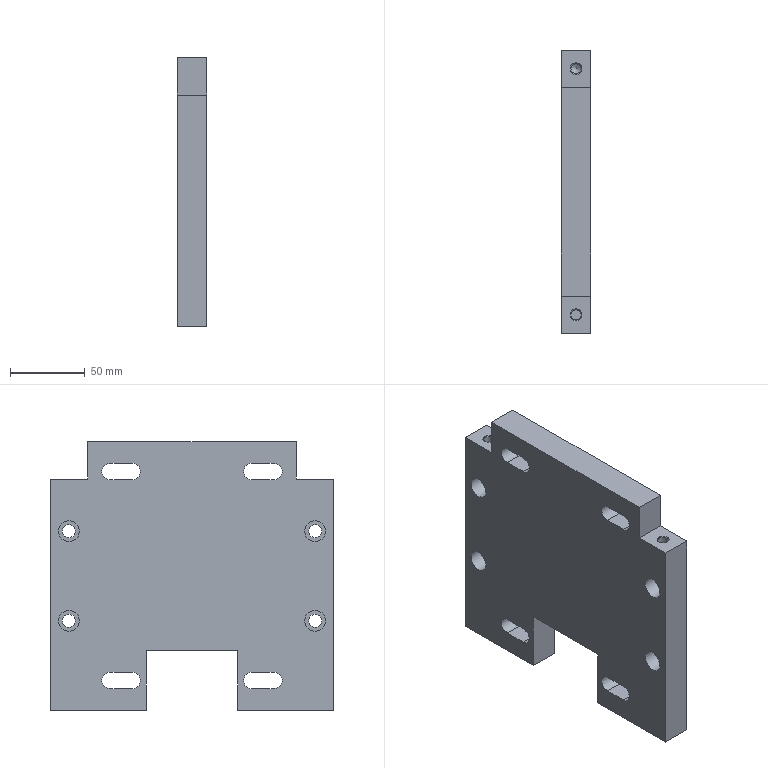Part | STEP file | 冲床-300配套压波_id982_x_t | 1 solid | 48 faces | box 20 x 190 x 180 mm | volume 579376 mm3 | plane 27 | cylinder 18 | cone 3 | commonest cylinder face diameters 11 x8 8.7 x4 14 x4 6.8 x2
STEP:
#1=CARTESIAN_POINT('',(1935.,-95.,-365.));
#2=VERTEX_POINT('',#1);
#3=CARTESIAN_POINT('',(1935.,-30.5,-365.));
#4=VERTEX_POINT('',#3);
#5=CARTESIAN_POINT('',(1935.,-100.,-365.));
#6=DIRECTION('',(0.,1.,0.));
#7=VECTOR('',#6,1.);
#8=LINE('',#5,#7);
#9=EDGE_CURVE('',#2,#4,#8,.T.);
#10=ORIENTED_EDGE('',*,*,#9,.T.);
#11=CARTESIAN_POINT('',(1955.,-30.5,-365.));
#12=VERTEX_POINT('',#11);
#13=CARTESIAN_POINT('',(1935.,-30.5,-365.));
#14=DIRECTION('',(1.,0.,0.));
#15=VECTOR('',#14,1.);
#16=LINE('',#13,#15);
#17=EDGE_CURVE('',#4,#12,#16,.T.);
#18=ORIENTED_EDGE('',*,*,#17,.T.);
#19=CARTESIAN_POINT('',(1955.,-95.,-365.));
#20=VERTEX_POINT('',#19);
#21=CARTESIAN_POINT('',(1955.,-100.,-365.));
#22=DIRECTION('',(0.,1.,0.));
#23=VECTOR('',#22,1.);
#24=LINE('',#21,#23);
#25=EDGE_CURVE('',#20,#12,#24,.T.);
#26=ORIENTED_EDGE('',*,*,#25,.F.);
#27=CARTESIAN_POINT('',(1935.,-95.,-365.));
#28=DIRECTION('',(1.,0.,0.));
#29=VECTOR('',#28,1.);
#30=LINE('',#27,#29);
#31=EDGE_CURVE('',#2,#20,#30,.T.);
#32=ORIENTED_EDGE('',*,*,#31,.F.);
#33=EDGE_LOOP('',(#10,#18,#26,#32));
#34=FACE_OUTER_BOUND('',#33,.T.);
#35=CARTESIAN_POINT('',(1935.,-100.,-365.));
#36=DIRECTION('',(0.,0.,-1.));
#37=DIRECTION('',(0.,1.,0.));
#38=AXIS2_PLACEMENT_3D('',#35,#36,#37);
#39=PLANE('',#38);
#40=ADVANCED_FACE('',(#34),#39,.T.);
#41=CARTESIAN_POINT('',(1941.6,-82.5,-230.));
#42=VERTEX_POINT('',#41);
#43=CARTESIAN_POINT('',(1945.,-82.5,-230.));
#44=DIRECTION('',(0.,0.,1.));
#45=DIRECTION('',(-1.,0.,0.));
#46=AXIS2_PLACEMENT_3D('',#43,#44,#45);
#47=CIRCLE('',#46,3.4);
#48=EDGE_CURVE('',#42,#42,#47,.T.);
#49=ORIENTED_EDGE('',*,*,#48,.T.);
#50=EDGE_LOOP('',(#49));
#51=FACE_OUTER_BOUND('',#50,.T.);
#52=CARTESIAN_POINT('',(1945.,-82.5,-230.));
#53=DIRECTION('',(0.,0.,-1.));
#54=DIRECTION('',(-1.,0.,0.));
#55=AXIS2_PLACEMENT_3D('',#52,#53,#54);
#56=PLANE('',#55);
#57=ADVANCED_FACE('',(#51),#56,.F.);
#58=CARTESIAN_POINT('',(1941.6,82.5,-230.));
#59=VERTEX_POINT('',#58);
#60=CARTESIAN_POINT('',(1945.,82.5,-230.));
#61=DIRECTION('',(0.,0.,1.));
#62=DIRECTION('',(-1.,0.,0.));
#63=AXIS2_PLACEMENT_3D('',#60,#61,#62);
#64=CIRCLE('',#63,3.4);
#65=EDGE_CURVE('',#59,#59,#64,.T.);
#66=ORIENTED_EDGE('',*,*,#65,.T.);
#67=EDGE_LOOP('',(#66));
#68=FACE_BOUND('',#67,.T.);
#69=CARTESIAN_POINT('',(1945.,82.5,-232.043));
#70=VERTEX_POINT('',#69);
#71=VERTEX_LOOP('',#70);
#72=FACE_BOUND('',#71,.T.);
#73=CARTESIAN_POINT('',(1945.,82.5,-230.));
#74=DIRECTION('',(0.,0.,1.));
#75=DIRECTION('',(1.,0.,0.));
#76=AXIS2_PLACEMENT_3D('',#73,#74,#75);
#77=CONICAL_SURFACE('',#76,3.4,59.);
#78=ADVANCED_FACE('',(#68,#72),#77,.F.);
#79=CARTESIAN_POINT('',(1941.6,-82.5,-210.6));
#80=VERTEX_POINT('',#79);
#81=CARTESIAN_POINT('',(1945.,-82.5,-210.6));
#82=DIRECTION('',(0.,0.,1.));
#83=DIRECTION('',(-1.,0.,0.));
#84=AXIS2_PLACEMENT_3D('',#81,#82,#83);
#85=CIRCLE('',#84,3.4);
#86=EDGE_CURVE('',#80,#80,#85,.T.);
#87=ORIENTED_EDGE('',*,*,#86,.T.);
#88=EDGE_LOOP('',(#87));
#89=FACE_BOUND('',#88,.T.);
#90=ORIENTED_EDGE('',*,*,#48,.F.);
#91=EDGE_LOOP('',(#90));
#92=FACE_BOUND('',#91,.T.);
#93=CARTESIAN_POINT('',(1945.,-82.5,-210.));
#94=DIRECTION('',(0.,0.,-1.));
#95=DIRECTION('',(-1.,0.,0.));
#96=AXIS2_PLACEMENT_3D('',#93,#94,#95);
#97=CYLINDRICAL_SURFACE('',#96,3.4);
#98=ADVANCED_FACE('',(#89,#92),#97,.F.);
#99=CARTESIAN_POINT('',(1941.6,82.5,-210.6));
#100=VERTEX_POINT('',#99);
#101=CARTESIAN_POINT('',(1945.,82.5,-210.6));
#102=DIRECTION('',(0.,0.,1.));
#103=DIRECTION('',(-1.,0.,0.));
#104=AXIS2_PLACEMENT_3D('',#101,#102,#103);
#105=CIRCLE('',#104,3.4);
#106=EDGE_CURVE('',#100,#100,#105,.T.);
#107=ORIENTED_EDGE('',*,*,#106,.T.);
#108=EDGE_LOOP('',(#107));
#109=FACE_BOUND('',#108,.T.);
#110=ORIENTED_EDGE('',*,*,#65,.F.);
#111=EDGE_LOOP('',(#110));
#112=FACE_BOUND('',#111,.T.);
#113=CARTESIAN_POINT('',(1945.,82.5,-210.));
#114=DIRECTION('',(0.,0.,-1.));
#115=DIRECTION('',(-1.,0.,0.));
#116=AXIS2_PLACEMENT_3D('',#113,#114,#115);
#117=CYLINDRICAL_SURFACE('',#116,3.4);
#118=ADVANCED_FACE('',(#109,#112),#117,.F.);
#119=ORIENTED_EDGE('',*,*,#86,.F.);
#120=EDGE_LOOP('',(#119));
#121=FACE_BOUND('',#120,.T.);
#122=CARTESIAN_POINT('',(1941.,-82.5,-210.));
#123=VERTEX_POINT('',#122);
#124=CARTESIAN_POINT('',(1945.,-82.5,-210.));
#125=DIRECTION('',(0.,0.,-1.));
#126=DIRECTION('',(-1.,0.,0.));
#127=AXIS2_PLACEMENT_3D('',#124,#125,#126);
#128=CIRCLE('',#127,4.);
#129=EDGE_CURVE('',#123,#123,#128,.T.);
#130=ORIENTED_EDGE('',*,*,#129,.F.);
#131=EDGE_LOOP('',(#130));
#132=FACE_BOUND('',#131,.T.);
#133=CARTESIAN_POINT('',(1945.,-82.5,-210.));
#134=DIRECTION('',(0.,0.,1.));
#135=DIRECTION('',(1.,0.,0.));
#136=AXIS2_PLACEMENT_3D('',#133,#134,#135);
#137=CONICAL_SURFACE('',#136,4.,45.);
#138=ADVANCED_FACE('',(#121,#132),#137,.F.);
#139=ORIENTED_EDGE('',*,*,#106,.F.);
#140=EDGE_LOOP('',(#139));
#141=FACE_BOUND('',#140,.T.);
#142=CARTESIAN_POINT('',(1941.,82.5,-210.));
#143=VERTEX_POINT('',#142);
#144=CARTESIAN_POINT('',(1945.,82.5,-210.));
#145=DIRECTION('',(0.,0.,-1.));
#146=DIRECTION('',(-1.,0.,0.));
#147=AXIS2_PLACEMENT_3D('',#144,#145,#146);
#148=CIRCLE('',#147,4.);
#149=EDGE_CURVE('',#143,#143,#148,.T.);
#150=ORIENTED_EDGE('',*,*,#149,.F.);
#151=EDGE_LOOP('',(#150));
#152=FACE_BOUND('',#151,.T.);
#153=CARTESIAN_POINT('',(1945.,82.5,-210.));
#154=DIRECTION('',(0.,0.,1.));
#155=DIRECTION('',(1.,0.,0.));
#156=AXIS2_PLACEMENT_3D('',#153,#154,#155);
#157=CONICAL_SURFACE('',#156,4.,45.);
#158=ADVANCED_FACE('',(#141,#152),#157,.F.);
#159=CARTESIAN_POINT('',(1945.,82.5,-249.35));
#160=VERTEX_POINT('',#159);
#161=CARTESIAN_POINT('',(1945.,82.5,-245.));
#162=DIRECTION('',(-1.,0.,0.));
#163=DIRECTION('',(0.,0.,-1.));
#164=AXIS2_PLACEMENT_3D('',#161,#162,#163);
#165=CIRCLE('',#164,4.35);
#166=EDGE_CURVE('',#160,#160,#165,.T.);
#167=ORIENTED_EDGE('',*,*,#166,.F.);
#168=EDGE_LOOP('',(#167));
#169=FACE_BOUND('',#168,.T.);
#170=CARTESIAN_POINT('',(1945.,82.5,-252.));
#171=VERTEX_POINT('',#170);
#172=CARTESIAN_POINT('',(1945.,82.5,-245.));
#173=DIRECTION('',(-1.,0.,0.));
#174=DIRECTION('',(0.,0.,-1.));
#175=AXIS2_PLACEMENT_3D('',#172,#173,#174);
#176=CIRCLE('',#175,7.);
#177=EDGE_CURVE('',#171,#171,#176,.T.);
#178=ORIENTED_EDGE('',*,*,#177,.T.);
#179=EDGE_LOOP('',(#178));
#180=FACE_BOUND('',#179,.T.);
#181=CARTESIAN_POINT('',(1945.,82.5,-245.));
#182=DIRECTION('',(1.,0.,0.));
#183=DIRECTION('',(0.,0.,-1.));
#184=AXIS2_PLACEMENT_3D('',#181,#182,#183);
#185=PLANE('',#184);
#186=ADVANCED_FACE('',(#169,#180),#185,.F.);
#187=CARTESIAN_POINT('',(1945.,82.5,-309.35));
#188=VERTEX_POINT('',#187);
#189=CARTESIAN_POINT('',(1945.,82.5,-305.));
#190=DIRECTION('',(-1.,0.,0.));
#191=DIRECTION('',(0.,0.,-1.));
#192=AXIS2_PLACEMENT_3D('',#189,#190,#191);
#193=CIRCLE('',#192,4.35);
#194=EDGE_CURVE('',#188,#188,#193,.T.);
#195=ORIENTED_EDGE('',*,*,#194,.F.);
#196=EDGE_LOOP('',(#195));
#197=FACE_BOUND('',#196,.T.);
#198=CARTESIAN_POINT('',(1945.,82.5,-312.));
#199=VERTEX_POINT('',#198);
#200=CARTESIAN_POINT('',(1945.,82.5,-305.));
#201=DIRECTION('',(-1.,0.,0.));
#202=DIRECTION('',(0.,0.,-1.));
#203=AXIS2_PLACEMENT_3D('',#200,#201,#202);
#204=CIRCLE('',#203,7.);
#205=EDGE_CURVE('',#199,#199,#204,.T.);
#206=ORIENTED_EDGE('',*,*,#205,.T.);
#207=EDGE_LOOP('',(#206));
#208=FACE_BOUND('',#207,.T.);
#209=CARTESIAN_POINT('',(1945.,82.5,-305.));
#210=DIRECTION('',(1.,0.,0.));
#211=DIRECTION('',(0.,0.,-1.));
#212=AXIS2_PLACEMENT_3D('',#209,#210,#211);
#213=PLANE('',#212);
#214=ADVANCED_FACE('',(#197,#208),#213,.F.);
#215=CARTESIAN_POINT('',(1945.,-82.5,-309.35));
#216=VERTEX_POINT('',#215);
#217=CARTESIAN_POINT('',(1945.,-82.5,-305.));
#218=DIRECTION('',(-1.,0.,0.));
#219=DIRECTION('',(0.,0.,-1.));
#220=AXIS2_PLACEMENT_3D('',#217,#218,#219);
#221=CIRCLE('',#220,4.35);
#222=EDGE_CURVE('',#216,#216,#221,.T.);
#223=ORIENTED_EDGE('',*,*,#222,.F.);
#224=EDGE_LOOP('',(#223));
#225=FACE_BOUND('',#224,.T.);
#226=CARTESIAN_POINT('',(1945.,-82.5,-312.));
#227=VERTEX_POINT('',#226);
#228=CARTESIAN_POINT('',(1945.,-82.5,-305.));
#229=DIRECTION('',(-1.,0.,0.));
#230=DIRECTION('',(0.,0.,-1.));
#231=AXIS2_PLACEMENT_3D('',#228,#229,#230);
#232=CIRCLE('',#231,7.);
#233=EDGE_CURVE('',#227,#227,#232,.T.);
#234=ORIENTED_EDGE('',*,*,#233,.T.);
#235=EDGE_LOOP('',(#234));
#236=FACE_BOUND('',#235,.T.);
#237=CARTESIAN_POINT('',(1945.,-82.5,-305.));
#238=DIRECTION('',(1.,0.,0.));
#239=DIRECTION('',(0.,0.,-1.));
#240=AXIS2_PLACEMENT_3D('',#237,#238,#239);
#241=PLANE('',#240);
#242=ADVANCED_FACE('',(#225,#236),#241,.F.);
#243=CARTESIAN_POINT('',(1945.,-82.5,-249.35));
#244=VERTEX_POINT('',#243);
#245=CARTESIAN_POINT('',(1945.,-82.5,-245.));
#246=DIRECTION('',(-1.,0.,0.));
#247=DIRECTION('',(0.,0.,-1.));
#248=AXIS2_PLACEMENT_3D('',#245,#246,#247);
#249=CIRCLE('',#248,4.35);
#250=EDGE_CURVE('',#244,#244,#249,.T.);
#251=ORIENTED_EDGE('',*,*,#250,.F.);
#252=EDGE_LOOP('',(#251));
#253=FACE_BOUND('',#252,.T.);
#254=CARTESIAN_POINT('',(1945.,-82.5,-252.));
#255=VERTEX_POINT('',#254);
#256=CARTESIAN_POINT('',(1945.,-82.5,-245.));
#257=DIRECTION('',(-1.,0.,0.));
#258=DIRECTION('',(0.,0.,-1.));
#259=AXIS2_PLACEMENT_3D('',#256,#257,#258);
#260=CIRCLE('',#259,7.);
#261=EDGE_CURVE('',#255,#255,#260,.T.);
#262=ORIENTED_EDGE('',*,*,#261,.T.);
#263=EDGE_LOOP('',(#262));
#264=FACE_BOUND('',#263,.T.);
#265=CARTESIAN_POINT('',(1945.,-82.5,-245.));
#266=DIRECTION('',(1.,0.,0.));
#267=DIRECTION('',(0.,0.,-1.));
#268=AXIS2_PLACEMENT_3D('',#265,#266,#267);
#269=PLANE('',#268);
#270=ADVANCED_FACE('',(#253,#264),#269,.F.);
#271=CARTESIAN_POINT('',(1955.,-40.,-339.5));
#272=VERTEX_POINT('',#271);
#273=CARTESIAN_POINT('',(1955.,-55.,-339.5));
#274=VERTEX_POINT('',#273);
#275=CARTESIAN_POINT('',(1955.,-100.,-339.5));
#276=DIRECTION('',(0.,-1.,0.));
#277=VECTOR('',#276,1.);
#278=LINE('',#275,#277);
#279=EDGE_CURVE('',#272,#274,#278,.T.);
#280=ORIENTED_EDGE('',*,*,#279,.T.);
#281=CARTESIAN_POINT('',(1935.,-55.,-339.5));
#282=VERTEX_POINT('',#281);
#283=CARTESIAN_POINT('',(1785.,-55.,-339.5));
#284=DIRECTION('',(-1.,0.,0.));
#285=VECTOR('',#284,1.);
#286=LINE('',#283,#285);
#287=EDGE_CURVE('',#274,#282,#286,.T.);
#288=ORIENTED_EDGE('',*,*,#287,.T.);
#289=CARTESIAN_POINT('',(1935.,-40.,-339.5));
#290=VERTEX_POINT('',#289);
#291=CARTESIAN_POINT('',(1935.,-100.,-339.5));
#292=DIRECTION('',(0.,-1.,0.));
#293=VECTOR('',#292,1.);
#294=LINE('',#291,#293);
#295=EDGE_CURVE('',#290,#282,#294,.T.);
#296=ORIENTED_EDGE('',*,*,#295,.F.);
#297=CARTESIAN_POINT('',(1785.,-40.,-339.5));
#298=DIRECTION('',(-1.,0.,0.));
#299=VECTOR('',#298,1.);
#300=LINE('',#297,#299);
#301=EDGE_CURVE('',#272,#290,#300,.T.);
#302=ORIENTED_EDGE('',*,*,#301,.F.);
#303=EDGE_LOOP('',(#280,#288,#296,#302));
#304=FACE_OUTER_BOUND('',#303,.T.);
#305=CARTESIAN_POINT('',(1785.,-30.,-339.5));
#306=DIRECTION('',(0.,0.,1.));
#307=DIRECTION('',(1.,0.,0.));
#308=AXIS2_PLACEMENT_3D('',#305,#306,#307);
#309=PLANE('',#308);
#310=ADVANCED_FACE('',(#304),#309,.F.);
#311=CARTESIAN_POINT('',(1955.,-55.,-350.5));
#312=VERTEX_POINT('',#311);
#313=CARTESIAN_POINT('',(1955.,-55.,-345.));
#314=DIRECTION('',(1.,0.,0.));
#315=DIRECTION('',(0.,0.,-1.));
#316=AXIS2_PLACEMENT_3D('',#313,#314,#315);
#317=CIRCLE('',#316,5.5);
#318=EDGE_CURVE('',#274,#312,#317,.T.);
#319=ORIENTED_EDGE('',*,*,#318,.T.);
#320=CARTESIAN_POINT('',(1935.,-55.,-350.5));
#321=VERTEX_POINT('',#320);
#322=CARTESIAN_POINT('',(1785.,-55.,-350.5));
#323=DIRECTION('',(-1.,0.,0.));
#324=VECTOR('',#323,1.);
#325=LINE('',#322,#324);
#326=EDGE_CURVE('',#312,#321,#325,.T.);
#327=ORIENTED_EDGE('',*,*,#326,.T.);
#328=CARTESIAN_POINT('',(1935.,-55.,-345.));
#329=DIRECTION('',(1.,0.,0.));
#330=DIRECTION('',(0.,0.,-1.));
#331=AXIS2_PLACEMENT_3D('',#328,#329,#330);
#332=CIRCLE('',#331,5.5);
#333=EDGE_CURVE('',#282,#321,#332,.T.);
#334=ORIENTED_EDGE('',*,*,#333,.F.);
#335=ORIENTED_EDGE('',*,*,#287,.F.);
#336=EDGE_LOOP('',(#319,#327,#334,#335));
#337=FACE_OUTER_BOUND('',#336,.T.);
#338=CARTESIAN_POINT('',(1785.,-55.,-345.));
#339=DIRECTION('',(1.,0.,0.));
#340=DIRECTION('',(0.,0.,-1.));
#341=AXIS2_PLACEMENT_3D('',#338,#339,#340);
#342=CYLINDRICAL_SURFACE('',#341,5.5);
#343=ADVANCED_FACE('',(#337),#342,.F.);
#344=CARTESIAN_POINT('',(1955.,-40.,-350.5));
#345=VERTEX_POINT('',#344);
#346=CARTESIAN_POINT('',(1955.,-100.,-350.5));
#347=DIRECTION('',(0.,-1.,0.));
#348=VECTOR('',#347,1.);
#349=LINE('',#346,#348);
#350=EDGE_CURVE('',#345,#312,#349,.T.);
#351=ORIENTED_EDGE('',*,*,#350,.F.);
#352=CARTESIAN_POINT('',(1935.,-40.,-350.5));
#353=VERTEX_POINT('',#352);
#354=CARTESIAN_POINT('',(1785.,-40.,-350.5));
#355=DIRECTION('',(-1.,0.,0.));
#356=VECTOR('',#355,1.);
#357=LINE('',#354,#356);
#358=EDGE_CURVE('',#345,#353,#357,.T.);
#359=ORIENTED_EDGE('',*,*,#358,.T.);
#360=CARTESIAN_POINT('',(1935.,-100.,-350.5));
#361=DIRECTION('',(0.,1.,0.));
#362=VECTOR('',#361,1.);
#363=LINE('',#360,#362);
#364=EDGE_CURVE('',#321,#353,#363,.T.);
#365=ORIENTED_EDGE('',*,*,#364,.F.);
#366=ORIENTED_EDGE('',*,*,#326,.F.);
#367=EDGE_LOOP('',(#351,#359,#365,#366));
#368=FACE_OUTER_BOUND('',#367,.T.);
#369=CARTESIAN_POINT('',(1785.,-70.,-350.5));
#370=DIRECTION('',(0.,0.,-1.));
#371=DIRECTION('',(-1.,0.,0.));
#372=AXIS2_PLACEMENT_3D('',#369,#370,#371);
#373=PLANE('',#372);
#374=ADVANCED_FACE('',(#368),#373,.F.);
#375=CARTESIAN_POINT('',(1955.,-40.,-345.));
#376=DIRECTION('',(1.,0.,0.));
#377=DIRECTION('',(0.,0.,-1.));
#378=AXIS2_PLACEMENT_3D('',#375,#376,#377);
#379=CIRCLE('',#378,5.5);
#380=EDGE_CURVE('',#345,#272,#379,.T.);
#381=ORIENTED_EDGE('',*,*,#380,.T.);
#382=ORIENTED_EDGE('',*,*,#301,.T.);
#383=CARTESIAN_POINT('',(1935.,-40.,-345.));
#384=DIRECTION('',(1.,0.,0.));
#385=DIRECTION('',(0.,0.,-1.));
#386=AXIS2_PLACEMENT_3D('',#383,#384,#385);
#387=CIRCLE('',#386,5.5);
#388=EDGE_CURVE('',#353,#290,#387,.T.);
#389=ORIENTED_EDGE('',*,*,#388,.F.);
#390=ORIENTED_EDGE('',*,*,#358,.F.);
#391=EDGE_LOOP('',(#381,#382,#389,#390));
#392=FACE_OUTER_BOUND('',#391,.T.);
#393=CARTESIAN_POINT('',(1785.,-40.,-345.));
#394=DIRECTION('',(1.,0.,0.));
#395=DIRECTION('',(0.,0.,-1.));
#396=AXIS2_PLACEMENT_3D('',#393,#394,#395);
#397=CYLINDRICAL_SURFACE('',#396,5.5);
#398=ADVANCED_FACE('',(#392),#397,.F.);
#399=CARTESIAN_POINT('',(1955.,55.,-210.5));
#400=VERTEX_POINT('',#399);
#401=CARTESIAN_POINT('',(1955.,55.,-199.5));
#402=VERTEX_POINT('',#401);
#403=CARTESIAN_POINT('',(1955.,55.,-205.));
#404=DIRECTION('',(1.,0.,0.));
#405=DIRECTION('',(0.,0.,-1.));
#406=AXIS2_PLACEMENT_3D('',#403,#404,#405);
#407=CIRCLE('',#406,5.5);
#408=EDGE_CURVE('',#400,#402,#407,.T.);
#409=ORIENTED_EDGE('',*,*,#408,.T.);
#410=CARTESIAN_POINT('',(1935.,55.,-199.5));
#411=VERTEX_POINT('',#410);
#412=CARTESIAN_POINT('',(1785.,55.,-199.5));
#413=DIRECTION('',(-1.,0.,0.));
#414=VECTOR('',#413,1.);
#415=LINE('',#412,#414);
#416=EDGE_CURVE('',#402,#411,#415,.T.);
#417=ORIENTED_EDGE('',*,*,#416,.T.);
#418=CARTESIAN_POINT('',(1935.,55.,-210.5));
#419=VERTEX_POINT('',#418);
#420=CARTESIAN_POINT('',(1935.,55.,-205.));
#421=DIRECTION('',(1.,0.,0.));
#422=DIRECTION('',(0.,0.,-1.));
#423=AXIS2_PLACEMENT_3D('',#420,#421,#422);
#424=CIRCLE('',#423,5.5);
#425=EDGE_CURVE('',#419,#411,#424,.T.);
#426=ORIENTED_EDGE('',*,*,#425,.F.);
#427=CARTESIAN_POINT('',(1785.,55.,-210.5));
#428=DIRECTION('',(-1.,0.,0.));
#429=VECTOR('',#428,1.);
#430=LINE('',#427,#429);
#431=EDGE_CURVE('',#400,#419,#430,.T.);
#432=ORIENTED_EDGE('',*,*,#431,.F.);
#433=EDGE_LOOP('',(#409,#417,#426,#432));
#434=FACE_OUTER_BOUND('',#433,.T.);
#435=CARTESIAN_POINT('',(1785.,55.,-205.));
#436=DIRECTION('',(1.,0.,0.));
#437=DIRECTION('',(0.,0.,1.));
#438=AXIS2_PLACEMENT_3D('',#435,#436,#437);
#439=CYLINDRICAL_SURFACE('',#438,5.5);
#440=ADVANCED_FACE('',(#434),#439,.F.);
#441=CARTESIAN_POINT('',(1955.,40.,-199.5));
#442=VERTEX_POINT('',#441);
#443=CARTESIAN_POINT('',(1955.,-100.,-199.5));
#444=DIRECTION('',(0.,-1.,0.));
#445=VECTOR('',#444,1.);
#446=LINE('',#443,#445);
#447=EDGE_CURVE('',#402,#442,#446,.T.);
#448=ORIENTED_EDGE('',*,*,#447,.T.);
#449=CARTESIAN_POINT('',(1935.,40.,-199.5));
#450=VERTEX_POINT('',#449);
#451=CARTESIAN_POINT('',(1785.,40.,-199.5));
#452=DIRECTION('',(-1.,0.,0.));
#453=VECTOR('',#452,1.);
#454=LINE('',#451,#453);
#455=EDGE_CURVE('',#442,#450,#454,.T.);
#456=ORIENTED_EDGE('',*,*,#455,.T.);
#457=CARTESIAN_POINT('',(1935.,-100.,-199.5));
#458=DIRECTION('',(0.,-1.,0.));
#459=VECTOR('',#458,1.);
#460=LINE('',#457,#459);
#461=EDGE_CURVE('',#411,#450,#460,.T.);
#462=ORIENTED_EDGE('',*,*,#461,.F.);
#463=ORIENTED_EDGE('',*,*,#416,.F.);
#464=EDGE_LOOP('',(#448,#456,#462,#463));
#465=FACE_OUTER_BOUND('',#464,.T.);
#466=CARTESIAN_POINT('',(1785.,70.,-199.5));
#467=DIRECTION('',(0.,0.,1.));
#468=DIRECTION('',(-1.,0.,0.));
#469=AXIS2_PLACEMENT_3D('',#466,#467,#468);
#470=PLANE('',#469);
#471=ADVANCED_FACE('',(#465),#470,.F.);
#472=CARTESIAN_POINT('',(1955.,40.,-210.5));
#473=VERTEX_POINT('',#472);
#474=CARTESIAN_POINT('',(1955.,40.,-205.));
#475=DIRECTION('',(-1.,0.,0.));
#476=DIRECTION('',(0.,0.,-1.));
#477=AXIS2_PLACEMENT_3D('',#474,#475,#476);
#478=CIRCLE('',#477,5.5);
#479=EDGE_CURVE('',#473,#442,#478,.T.);
#480=ORIENTED_EDGE('',*,*,#479,.F.);
#481=CARTESIAN_POINT('',(1935.,40.,-210.5));
#482=VERTEX_POINT('',#481);
#483=CARTESIAN_POINT('',(1785.,40.,-210.5));
#484=DIRECTION('',(-1.,0.,0.));
#485=VECTOR('',#484,1.);
#486=LINE('',#483,#485);
#487=EDGE_CURVE('',#473,#482,#486,.T.);
#488=ORIENTED_EDGE('',*,*,#487,.T.);
#489=CARTESIAN_POINT('',(1935.,40.,-205.));
#490=DIRECTION('',(1.,0.,0.));
#491=DIRECTION('',(0.,0.,-1.));
#492=AXIS2_PLACEMENT_3D('',#489,#490,#491);
#493=CIRCLE('',#492,5.5);
#494=EDGE_CURVE('',#450,#482,#493,.T.);
#495=ORIENTED_EDGE('',*,*,#494,.F.);
#496=ORIENTED_EDGE('',*,*,#455,.F.);
#497=EDGE_LOOP('',(#480,#488,#495,#496));
#498=FACE_OUTER_BOUND('',#497,.T.);
#499=CARTESIAN_POINT('',(1785.,40.,-205.));
#500=DIRECTION('',(1.,0.,0.));
#501=DIRECTION('',(0.,0.,1.));
#502=AXIS2_PLACEMENT_3D('',#499,#500,#501);
#503=CYLINDRICAL_SURFACE('',#502,5.5);
#504=ADVANCED_FACE('',(#498),#503,.F.);
#505=CARTESIAN_POINT('',(1955.,-100.,-210.5));
#506=DIRECTION('',(0.,1.,0.));
#507=VECTOR('',#506,1.);
#508=LINE('',#505,#507);
#509=EDGE_CURVE('',#473,#400,#508,.T.);
#510=ORIENTED_EDGE('',*,*,#509,.T.);
#511=ORIENTED_EDGE('',*,*,#431,.T.);
#512=CARTESIAN_POINT('',(1935.,-100.,-210.5));
#513=DIRECTION('',(0.,1.,0.));
#514=VECTOR('',#513,1.);
#515=LINE('',#512,#514);
#516=EDGE_CURVE('',#482,#419,#515,.T.);
#517=ORIENTED_EDGE('',*,*,#516,.F.);
#518=ORIENTED_EDGE('',*,*,#487,.F.);
#519=EDGE_LOOP('',(#510,#511,#517,#518));
#520=FACE_OUTER_BOUND('',#519,.T.);
#521=CARTESIAN_POINT('',(1785.,30.,-210.5));
#522=DIRECTION('',(0.,0.,-1.));
#523=DIRECTION('',(1.,0.,0.));
#524=AXIS2_PLACEMENT_3D('',#521,#522,#523);
#525=PLANE('',#524);
#526=ADVANCED_FACE('',(#520),#525,.F.);
#527=CARTESIAN_POINT('',(1955.,-55.,-210.5));
#528=VERTEX_POINT('',#527);
#529=CARTESIAN_POINT('',(1955.,-40.,-210.5));
#530=VERTEX_POINT('',#529);
#531=CARTESIAN_POINT('',(1955.,-100.,-210.5));
#532=DIRECTION('',(0.,1.,0.));
#533=VECTOR('',#532,1.);
#534=LINE('',#531,#533);
#535=EDGE_CURVE('',#528,#530,#534,.T.);
#536=ORIENTED_EDGE('',*,*,#535,.T.);
#537=CARTESIAN_POINT('',(1935.,-40.,-210.5));
#538=VERTEX_POINT('',#537);
#539=CARTESIAN_POINT('',(1785.,-40.,-210.5));
#540=DIRECTION('',(1.,0.,0.));
#541=VECTOR('',#540,1.);
#542=LINE('',#539,#541);
#543=EDGE_CURVE('',#538,#530,#542,.T.);
#544=ORIENTED_EDGE('',*,*,#543,.F.);
#545=CARTESIAN_POINT('',(1935.,-55.,-210.5));
#546=VERTEX_POINT('',#545);
#547=CARTESIAN_POINT('',(1935.,-100.,-210.5));
#548=DIRECTION('',(0.,1.,0.));
#549=VECTOR('',#548,1.);
#550=LINE('',#547,#549);
#551=EDGE_CURVE('',#546,#538,#550,.T.);
#552=ORIENTED_EDGE('',*,*,#551,.F.);
#553=CARTESIAN_POINT('',(1785.,-55.,-210.5));
#554=DIRECTION('',(1.,0.,0.));
#555=VECTOR('',#554,1.);
#556=LINE('',#553,#555);
#557=EDGE_CURVE('',#546,#528,#556,.T.);
#558=ORIENTED_EDGE('',*,*,#557,.T.);
#559=EDGE_LOOP('',(#536,#544,#552,#558));
#560=FACE_OUTER_BOUND('',#559,.T.);
#561=CARTESIAN_POINT('',(1785.,-30.,-210.5));
#562=DIRECTION('',(0.,0.,-1.));
#563=DIRECTION('',(1.,0.,0.));
#564=AXIS2_PLACEMENT_3D('',#561,#562,#563);
#565=PLANE('',#564);
#566=ADVANCED_FACE('',(#560),#565,.F.);
#567=CARTESIAN_POINT('',(1955.,-40.,-199.5));
#568=VERTEX_POINT('',#567);
#569=CARTESIAN_POINT('',(1955.,-40.,-205.));
#570=DIRECTION('',(1.,0.,0.));
#571=DIRECTION('',(0.,0.,-1.));
#572=AXIS2_PLACEMENT_3D('',#569,#570,#571);
#573=CIRCLE('',#572,5.5);
#574=EDGE_CURVE('',#530,#568,#573,.T.);
#575=ORIENTED_EDGE('',*,*,#574,.T.);
#576=CARTESIAN_POINT('',(1935.,-40.,-199.5));
#577=VERTEX_POINT('',#576);
#578=CARTESIAN_POINT('',(1785.,-40.,-199.5));
#579=DIRECTION('',(1.,0.,0.));
#580=VECTOR('',#579,1.);
#581=LINE('',#578,#580);
#582=EDGE_CURVE('',#577,#568,#581,.T.);
#583=ORIENTED_EDGE('',*,*,#582,.F.);
#584=CARTESIAN_POINT('',(1935.,-40.,-205.));
#585=DIRECTION('',(1.,0.,0.));
#586=DIRECTION('',(0.,0.,-1.));
#587=AXIS2_PLACEMENT_3D('',#584,#585,#586);
#588=CIRCLE('',#587,5.5);
#589=EDGE_CURVE('',#538,#577,#588,.T.);
#590=ORIENTED_EDGE('',*,*,#589,.F.);
#591=ORIENTED_EDGE('',*,*,#543,.T.);
#592=EDGE_LOOP('',(#575,#583,#590,#591));
#593=FACE_OUTER_BOUND('',#592,.T.);
#594=CARTESIAN_POINT('',(1785.,-40.,-205.));
#595=DIRECTION('',(1.,0.,0.));
#596=DIRECTION('',(0.,0.,1.));
#597=AXIS2_PLACEMENT_3D('',#594,#595,#596);
#598=CYLINDRICAL_SURFACE('',#597,5.5);
#599=ADVANCED_FACE('',(#593),#598,.F.);
#600=CARTESIAN_POINT('',(1955.,-55.,-199.5));
#601=VERTEX_POINT('',#600);
#602=CARTESIAN_POINT('',(1955.,-100.,-199.5));
#603=DIRECTION('',(0.,1.,0.));
#604=VECTOR('',#603,1.);
#605=LINE('',#602,#604);
#606=EDGE_CURVE('',#601,#568,#605,.T.);
#607=ORIENTED_EDGE('',*,*,#606,.F.);
#608=CARTESIAN_POINT('',(1935.,-55.,-199.5));
#609=VERTEX_POINT('',#608);
#610=CARTESIAN_POINT('',(1785.,-55.,-199.5));
#611=DIRECTION('',(1.,0.,0.));
#612=VECTOR('',#611,1.);
#613=LINE('',#610,#612);
#614=EDGE_CURVE('',#609,#601,#613,.T.);
#615=ORIENTED_EDGE('',*,*,#614,.F.);
#616=CARTESIAN_POINT('',(1935.,-100.,-199.5));
#617=DIRECTION('',(0.,-1.,0.));
#618=VECTOR('',#617,1.);
#619=LINE('',#616,#618);
#620=EDGE_CURVE('',#577,#609,#619,.T.);
#621=ORIENTED_EDGE('',*,*,#620,.F.);
#622=ORIENTED_EDGE('',*,*,#582,.T.);
#623=EDGE_LOOP('',(#607,#615,#621,#622));
#624=FACE_OUTER_BOUND('',#623,.T.);
#625=CARTESIAN_POINT('',(1785.,-70.,-199.5));
#626=DIRECTION('',(0.,0.,1.));
#627=DIRECTION('',(-1.,0.,0.));
#628=AXIS2_PLACEMENT_3D('',#625,#626,#627);
#629=PLANE('',#628);
#630=ADVANCED_FACE('',(#624),#629,.F.);
#631=CARTESIAN_POINT('',(1955.,-55.,-205.));
#632=DIRECTION('',(1.,0.,0.));
#633=DIRECTION('',(0.,0.,-1.));
#634=AXIS2_PLACEMENT_3D('',#631,#632,#633);
#635=CIRCLE('',#634,5.5);
#636=EDGE_CURVE('',#601,#528,#635,.T.);
#637=ORIENTED_EDGE('',*,*,#636,.T.);
#638=ORIENTED_EDGE('',*,*,#557,.F.);
#639=CARTESIAN_POINT('',(1935.,-55.,-205.));
#640=DIRECTION('',(1.,0.,0.));
#641=DIRECTION('',(0.,0.,-1.));
#642=AXIS2_PLACEMENT_3D('',#639,#640,#641);
#643=CIRCLE('',#642,5.5);
#644=EDGE_CURVE('',#609,#546,#643,.T.);
#645=ORIENTED_EDGE('',*,*,#644,.F.);
#646=ORIENTED_EDGE('',*,*,#614,.T.);
#647=EDGE_LOOP('',(#637,#638,#645,#646));
#648=FACE_OUTER_BOUND('',#647,.T.);
#649=CARTESIAN_POINT('',(1785.,-55.,-205.));
#650=DIRECTION('',(1.,0.,0.));
#651=DIRECTION('',(0.,0.,1.));
#652=AXIS2_PLACEMENT_3D('',#649,#650,#651);
#653=CYLINDRICAL_SURFACE('',#652,5.5);
#654=ADVANCED_FACE('',(#648),#653,.F.);
#655=ORIENTED_EDGE('',*,*,#129,.T.);
#656=EDGE_LOOP('',(#655));
#657=FACE_BOUND('',#656,.T.);
#658=CARTESIAN_POINT('',(1935.,-70.,-210.));
#659=VERTEX_POINT('',#658);
#660=CARTESIAN_POINT('',(1935.,-95.,-210.));
#661=VERTEX_POINT('',#660);
#662=CARTESIAN_POINT('',(1935.,-70.,-210.));
#663=DIRECTION('',(0.,-1.,0.));
#664=VECTOR('',#663,1.);
#665=LINE('',#662,#664);
#666=EDGE_CURVE('',#659,#661,#665,.T.);
#667=ORIENTED_EDGE('',*,*,#666,.T.);
#668=CARTESIAN_POINT('',(1955.,-95.,-210.));
#669=VERTEX_POINT('',#668);
#670=CARTESIAN_POINT('',(1935.,-95.,-210.));
#671=DIRECTION('',(-1.,0.,0.));
#672=VECTOR('',#671,1.);
#673=LINE('',#670,#672);
#674=EDGE_CURVE('',#669,#661,#673,.T.);
#675=ORIENTED_EDGE('',*,*,#674,.F.);
#676=CARTESIAN_POINT('',(1955.,-70.,-210.));
#677=VERTEX_POINT('',#676);
#678=CARTESIAN_POINT('',(1955.,-70.,-210.));
#679=DIRECTION('',(0.,-1.,0.));
#680=VECTOR('',#679,1.);
#681=LINE('',#678,#680);
#682=EDGE_CURVE('',#677,#669,#681,.T.);
#683=ORIENTED_EDGE('',*,*,#682,.F.);
#684=CARTESIAN_POINT('',(1955.,-70.,-210.));
#685=DIRECTION('',(-1.,0.,0.));
#686=VECTOR('',#685,1.);
#687=LINE('',#684,#686);
#688=EDGE_CURVE('',#677,#659,#687,.T.);
#689=ORIENTED_EDGE('',*,*,#688,.T.);
#690=EDGE_LOOP('',(#667,#675,#683,#689));
#691=FACE_BOUND('',#690,.T.);
#692=CARTESIAN_POINT('',(1955.,-70.,-210.));
#693=DIRECTION('',(0.,0.,-1.));
#694=DIRECTION('',(-1.,0.,0.));
#695=AXIS2_PLACEMENT_3D('',#692,#693,#694);
#696=PLANE('',#695);
#697=ADVANCED_FACE('',(#657,#691),#696,.F.);
#698=CARTESIAN_POINT('',(1955.,-70.,-185.));
#699=VERTEX_POINT('',#698);
#700=CARTESIAN_POINT('',(1935.,-70.,-185.));
#701=VERTEX_POINT('',#700);
#702=CARTESIAN_POINT('',(1935.,-70.,-185.));
#703=DIRECTION('',(-1.,0.,0.));
#704=VECTOR('',#703,1.);
#705=LINE('',#702,#704);
#706=EDGE_CURVE('',#699,#701,#705,.T.);
#707=ORIENTED_EDGE('',*,*,#706,.T.);
#708=CARTESIAN_POINT('',(1935.,-70.,-180.));
#709=DIRECTION('',(0.,0.,-1.));
#710=VECTOR('',#709,1.);
#711=LINE('',#708,#710);
#712=EDGE_CURVE('',#701,#659,#711,.T.);
#713=ORIENTED_EDGE('',*,*,#712,.T.);
#714=ORIENTED_EDGE('',*,*,#688,.F.);
#715=CARTESIAN_POINT('',(1955.,-70.,-225.));
#716=DIRECTION('',(0.,0.,-1.));
#717=VECTOR('',#716,1.);
#718=LINE('',#715,#717);
#719=EDGE_CURVE('',#699,#677,#718,.T.);
#720=ORIENTED_EDGE('',*,*,#719,.F.);
#721=EDGE_LOOP('',(#707,#713,#714,#720));
#722=FACE_OUTER_BOUND('',#721,.T.);
#723=CARTESIAN_POINT('',(2135.,-70.,-385.));
#724=DIRECTION('',(0.,-1.,0.));
#725=DIRECTION('',(0.,0.,-1.));
#726=AXIS2_PLACEMENT_3D('',#723,#724,#725);
#727=PLANE('',#726);
#728=ADVANCED_FACE('',(#722),#727,.T.);
#729=CARTESIAN_POINT('',(1955.,70.,-185.));
#730=VERTEX_POINT('',#729);
#731=CARTESIAN_POINT('',(1955.,-100.,-185.));
#732=DIRECTION('',(0.,1.,0.));
#733=VECTOR('',#732,1.);
#734=LINE('',#731,#733);
#735=EDGE_CURVE('',#699,#730,#734,.T.);
#736=ORIENTED_EDGE('',*,*,#735,.T.);
#737=CARTESIAN_POINT('',(1935.,70.,-185.));
#738=VERTEX_POINT('',#737);
#739=CARTESIAN_POINT('',(2135.,70.,-185.));
#740=DIRECTION('',(-1.,0.,0.));
#741=VECTOR('',#740,1.);
#742=LINE('',#739,#741);
#743=EDGE_CURVE('',#730,#738,#742,.T.);
#744=ORIENTED_EDGE('',*,*,#743,.T.);
#745=CARTESIAN_POINT('',(1935.,-100.,-185.));
#746=DIRECTION('',(0.,1.,0.));
#747=VECTOR('',#746,1.);
#748=LINE('',#745,#747);
#749=EDGE_CURVE('',#701,#738,#748,.T.);
#750=ORIENTED_EDGE('',*,*,#749,.F.);
#751=ORIENTED_EDGE('',*,*,#706,.F.);
#752=EDGE_LOOP('',(#736,#744,#750,#751));
#753=FACE_OUTER_BOUND('',#752,.T.);
#754=CARTESIAN_POINT('',(1935.,-100.,-185.));
#755=DIRECTION('',(0.,0.,-1.));
#756=DIRECTION('',(0.,1.,0.));
#757=AXIS2_PLACEMENT_3D('',#754,#755,#756);
#758=PLANE('',#757);
#759=ADVANCED_FACE('',(#753),#758,.F.);
#760=ORIENTED_EDGE('',*,*,#743,.F.);
#761=CARTESIAN_POINT('',(1955.,70.,-210.));
#762=VERTEX_POINT('',#761);
#763=CARTESIAN_POINT('',(1955.,70.,-225.));
#764=DIRECTION('',(0.,0.,1.));
#765=VECTOR('',#764,1.);
#766=LINE('',#763,#765);
#767=EDGE_CURVE('',#762,#730,#766,.T.);
#768=ORIENTED_EDGE('',*,*,#767,.F.);
#769=CARTESIAN_POINT('',(1935.,70.,-210.));
#770=VERTEX_POINT('',#769);
#771=CARTESIAN_POINT('',(2135.,70.,-210.));
#772=DIRECTION('',(-1.,0.,0.));
#773=VECTOR('',#772,1.);
#774=LINE('',#771,#773);
#775=EDGE_CURVE('',#762,#770,#774,.T.);
#776=ORIENTED_EDGE('',*,*,#775,.T.);
#777=CARTESIAN_POINT('',(1935.,70.,-180.));
#778=DIRECTION('',(0.,0.,-1.));
#779=VECTOR('',#778,1.);
#780=LINE('',#777,#779);
#781=EDGE_CURVE('',#738,#770,#780,.T.);
#782=ORIENTED_EDGE('',*,*,#781,.F.);
#783=EDGE_LOOP('',(#760,#768,#776,#782));
#784=FACE_OUTER_BOUND('',#783,.T.);
#785=CARTESIAN_POINT('',(2135.,70.,-385.));
#786=DIRECTION('',(0.,1.,0.));
#787=DIRECTION('',(0.,0.,-1.));
#788=AXIS2_PLACEMENT_3D('',#785,#786,#787);
#789=PLANE('',#788);
#790=ADVANCED_FACE('',(#784),#789,.T.);
#791=ORIENTED_EDGE('',*,*,#149,.T.);
#792=EDGE_LOOP('',(#791));
#793=FACE_BOUND('',#792,.T.);
#794=CARTESIAN_POINT('',(1935.,95.,-210.));
#795=VERTEX_POINT('',#794);
#796=CARTESIAN_POINT('',(1935.,70.,-210.));
#797=DIRECTION('',(0.,-1.,0.));
#798=VECTOR('',#797,1.);
#799=LINE('',#796,#798);
#800=EDGE_CURVE('',#795,#770,#799,.T.);
#801=ORIENTED_EDGE('',*,*,#800,.T.);
#802=ORIENTED_EDGE('',*,*,#775,.F.);
#803=CARTESIAN_POINT('',(1955.,95.,-210.));
#804=VERTEX_POINT('',#803);
#805=CARTESIAN_POINT('',(1955.,70.,-210.));
#806=DIRECTION('',(0.,-1.,0.));
#807=VECTOR('',#806,1.);
#808=LINE('',#805,#807);
#809=EDGE_CURVE('',#804,#762,#808,.T.);
#810=ORIENTED_EDGE('',*,*,#809,.F.);
#811=CARTESIAN_POINT('',(1955.,95.,-210.));
#812=DIRECTION('',(-1.,0.,0.));
#813=VECTOR('',#812,1.);
#814=LINE('',#811,#813);
#815=EDGE_CURVE('',#804,#795,#814,.T.);
#816=ORIENTED_EDGE('',*,*,#815,.T.);
#817=EDGE_LOOP('',(#801,#802,#810,#816));
#818=FACE_BOUND('',#817,.T.);
#819=CARTESIAN_POINT('',(1955.,70.,-210.));
#820=DIRECTION('',(0.,0.,-1.));
#821=DIRECTION('',(-1.,0.,0.));
#822=AXIS2_PLACEMENT_3D('',#819,#820,#821);
#823=PLANE('',#822);
#824=ADVANCED_FACE('',(#793,#818),#823,.F.);
#825=ORIENTED_EDGE('',*,*,#815,.F.);
#826=CARTESIAN_POINT('',(1955.,95.,-365.));
#827=VERTEX_POINT('',#826);
#828=CARTESIAN_POINT('',(1955.,95.,-225.));
#829=DIRECTION('',(0.,0.,-1.));
#830=VECTOR('',#829,1.);
#831=LINE('',#828,#830);
#832=EDGE_CURVE('',#804,#827,#831,.T.);
#833=ORIENTED_EDGE('',*,*,#832,.T.);
#834=CARTESIAN_POINT('',(1935.,95.,-365.));
#835=VERTEX_POINT('',#834);
#836=CARTESIAN_POINT('',(1935.,95.,-365.));
#837=DIRECTION('',(1.,0.,0.));
#838=VECTOR('',#837,1.);
#839=LINE('',#836,#838);
#840=EDGE_CURVE('',#835,#827,#839,.T.);
#841=ORIENTED_EDGE('',*,*,#840,.F.);
#842=CARTESIAN_POINT('',(1935.,95.,-180.));
#843=DIRECTION('',(0.,0.,-1.));
#844=VECTOR('',#843,1.);
#845=LINE('',#842,#844);
#846=EDGE_CURVE('',#795,#835,#845,.T.);
#847=ORIENTED_EDGE('',*,*,#846,.F.);
#848=EDGE_LOOP('',(#825,#833,#841,#847));
#849=FACE_OUTER_BOUND('',#848,.T.);
#850=CARTESIAN_POINT('',(1975.,95.,-70.));
#851=DIRECTION('',(0.,-1.,0.));
#852=DIRECTION('',(0.,0.,1.));
#853=AXIS2_PLACEMENT_3D('',#850,#851,#852);
#854=PLANE('',#853);
#855=ADVANCED_FACE('',(#849),#854,.F.);
#856=CARTESIAN_POINT('',(1955.,30.5,-365.));
#857=VERTEX_POINT('',#856);
#858=CARTESIAN_POINT('',(1955.,-100.,-365.));
#859=DIRECTION('',(0.,1.,0.));
#860=VECTOR('',#859,1.);
#861=LINE('',#858,#860);
#862=EDGE_CURVE('',#857,#827,#861,.T.);
#863=ORIENTED_EDGE('',*,*,#862,.F.);
#864=CARTESIAN_POINT('',(1935.,30.5,-365.));
#865=VERTEX_POINT('',#864);
#866=CARTESIAN_POINT('',(1935.,30.5,-365.));
#867=DIRECTION('',(-1.,0.,0.));
#868=VECTOR('',#867,1.);
#869=LINE('',#866,#868);
#870=EDGE_CURVE('',#857,#865,#869,.T.);
#871=ORIENTED_EDGE('',*,*,#870,.T.);
#872=CARTESIAN_POINT('',(1935.,-100.,-365.));
#873=DIRECTION('',(0.,1.,0.));
#874=VECTOR('',#873,1.);
#875=LINE('',#872,#874);
#876=EDGE_CURVE('',#865,#835,#875,.T.);
#877=ORIENTED_EDGE('',*,*,#876,.T.);
#878=ORIENTED_EDGE('',*,*,#840,.T.);
#879=EDGE_LOOP('',(#863,#871,#877,#878));
#880=FACE_OUTER_BOUND('',#879,.T.);
#881=CARTESIAN_POINT('',(1935.,-100.,-365.));
#882=DIRECTION('',(0.,0.,-1.));
#883=DIRECTION('',(0.,1.,0.));
#884=AXIS2_PLACEMENT_3D('',#881,#882,#883);
#885=PLANE('',#884);
#886=ADVANCED_FACE('',(#880),#885,.T.);
#887=CARTESIAN_POINT('',(1955.,-95.,-180.));
#888=DIRECTION('',(0.,0.,-1.));
#889=VECTOR('',#888,1.);
#890=LINE('',#887,#889);
#891=EDGE_CURVE('',#669,#20,#890,.T.);
#892=ORIENTED_EDGE('',*,*,#891,.F.);
#893=ORIENTED_EDGE('',*,*,#674,.T.);
#894=CARTESIAN_POINT('',(1935.,-95.,-180.));
#895=DIRECTION('',(0.,0.,-1.));
#896=VECTOR('',#895,1.);
#897=LINE('',#894,#896);
#898=EDGE_CURVE('',#661,#2,#897,.T.);
#899=ORIENTED_EDGE('',*,*,#898,.T.);
#900=ORIENTED_EDGE('',*,*,#31,.T.);
#901=EDGE_LOOP('',(#892,#893,#899,#900));
#902=FACE_OUTER_BOUND('',#901,.T.);
#903=CARTESIAN_POINT('',(1935.,-95.,-180.));
#904=DIRECTION('',(0.,-1.,0.));
#905=DIRECTION('',(0.,0.,-1.));
#906=AXIS2_PLACEMENT_3D('',#903,#904,#905);
#907=PLANE('',#906);
#908=ADVANCED_FACE('',(#902),#907,.T.);
#909=CARTESIAN_POINT('',(1955.,82.5,-249.35));
#910=VERTEX_POINT('',#909);
#911=CARTESIAN_POINT('',(1955.,82.5,-245.));
#912=DIRECTION('',(-1.,0.,0.));
#913=DIRECTION('',(0.,0.,-1.));
#914=AXIS2_PLACEMENT_3D('',#911,#912,#913);
#915=CIRCLE('',#914,4.35);
#916=EDGE_CURVE('',#910,#910,#915,.T.);
#917=ORIENTED_EDGE('',*,*,#916,.F.);
#918=EDGE_LOOP('',(#917));
#919=FACE_BOUND('',#918,.T.);
#920=ORIENTED_EDGE('',*,*,#166,.T.);
#921=EDGE_LOOP('',(#920));
#922=FACE_BOUND('',#921,.T.);
#923=CARTESIAN_POINT('',(1985.,82.5,-245.));
#924=DIRECTION('',(1.,0.,0.));
#925=DIRECTION('',(0.,0.,-1.));
#926=AXIS2_PLACEMENT_3D('',#923,#924,#925);
#927=CYLINDRICAL_SURFACE('',#926,4.35);
#928=ADVANCED_FACE('',(#919,#922),#927,.F.);
#929=CARTESIAN_POINT('',(1955.,82.5,-309.35));
#930=VERTEX_POINT('',#929);
#931=CARTESIAN_POINT('',(1955.,82.5,-305.));
#932=DIRECTION('',(-1.,0.,0.));
#933=DIRECTION('',(0.,0.,-1.));
#934=AXIS2_PLACEMENT_3D('',#931,#932,#933);
#935=CIRCLE('',#934,4.35);
#936=EDGE_CURVE('',#930,#930,#935,.T.);
#937=ORIENTED_EDGE('',*,*,#936,.F.);
#938=EDGE_LOOP('',(#937));
#939=FACE_BOUND('',#938,.T.);
#940=ORIENTED_EDGE('',*,*,#194,.T.);
#941=EDGE_LOOP('',(#940));
#942=FACE_BOUND('',#941,.T.);
#943=CARTESIAN_POINT('',(1985.,82.5,-305.));
#944=DIRECTION('',(1.,0.,0.));
#945=DIRECTION('',(0.,0.,-1.));
#946=AXIS2_PLACEMENT_3D('',#943,#944,#945);
#947=CYLINDRICAL_SURFACE('',#946,4.35);
#948=ADVANCED_FACE('',(#939,#942),#947,.F.);
#949=CARTESIAN_POINT('',(1955.,-82.5,-309.35));
#950=VERTEX_POINT('',#949);
#951=CARTESIAN_POINT('',(1955.,-82.5,-305.));
#952=DIRECTION('',(-1.,0.,0.));
#953=DIRECTION('',(0.,0.,-1.));
#954=AXIS2_PLACEMENT_3D('',#951,#952,#953);
#955=CIRCLE('',#954,4.35);
#956=EDGE_CURVE('',#950,#950,#955,.T.);
#957=ORIENTED_EDGE('',*,*,#956,.F.);
#958=EDGE_LOOP('',(#957));
#959=FACE_BOUND('',#958,.T.);
#960=ORIENTED_EDGE('',*,*,#222,.T.);
#961=EDGE_LOOP('',(#960));
#962=FACE_BOUND('',#961,.T.);
#963=CARTESIAN_POINT('',(1985.,-82.5,-305.));
#964=DIRECTION('',(1.,0.,0.));
#965=DIRECTION('',(0.,0.,-1.));
#966=AXIS2_PLACEMENT_3D('',#963,#964,#965);
#967=CYLINDRICAL_SURFACE('',#966,4.35);
#968=ADVANCED_FACE('',(#959,#962),#967,.F.);
#969=CARTESIAN_POINT('',(1955.,-82.5,-249.35));
#970=VERTEX_POINT('',#969);
#971=CARTESIAN_POINT('',(1955.,-82.5,-245.));
#972=DIRECTION('',(-1.,0.,0.));
#973=DIRECTION('',(0.,0.,-1.));
#974=AXIS2_PLACEMENT_3D('',#971,#972,#973);
#975=CIRCLE('',#974,4.35);
#976=EDGE_CURVE('',#970,#970,#975,.T.);
#977=ORIENTED_EDGE('',*,*,#976,.F.);
#978=EDGE_LOOP('',(#977));
#979=FACE_BOUND('',#978,.T.);
#980=ORIENTED_EDGE('',*,*,#250,.T.);
#981=EDGE_LOOP('',(#980));
#982=FACE_BOUND('',#981,.T.);
#983=CARTESIAN_POINT('',(1985.,-82.5,-245.));
#984=DIRECTION('',(1.,0.,0.));
#985=DIRECTION('',(0.,0.,-1.));
#986=AXIS2_PLACEMENT_3D('',#983,#984,#985);
#987=CYLINDRICAL_SURFACE('',#986,4.35);
#988=ADVANCED_FACE('',(#979,#982),#987,.F.);
#989=CARTESIAN_POINT('',(1955.,-30.5,-325.));
#990=VERTEX_POINT('',#989);
#991=CARTESIAN_POINT('',(1955.,-30.5,-225.));
#992=DIRECTION('',(0.,0.,-1.));
#993=VECTOR('',#992,1.);
#994=LINE('',#991,#993);
#995=EDGE_CURVE('',#990,#12,#994,.T.);
#996=ORIENTED_EDGE('',*,*,#995,.F.);
#997=CARTESIAN_POINT('',(1955.,30.5,-325.));
#998=VERTEX_POINT('',#997);
#999=CARTESIAN_POINT('',(1955.,0.,-325.));
#1000=DIRECTION('',(0.,-1.,0.));
#1001=VECTOR('',#1000,1.);
#1002=LINE('',#999,#1001);
#1003=EDGE_CURVE('',#998,#990,#1002,.T.);
#1004=ORIENTED_EDGE('',*,*,#1003,.F.);
#1005=CARTESIAN_POINT('',(1955.,30.5,-225.));
#1006=DIRECTION('',(0.,0.,1.));
#1007=VECTOR('',#1006,1.);
#1008=LINE('',#1005,#1007);
#1009=EDGE_CURVE('',#857,#998,#1008,.T.);
#1010=ORIENTED_EDGE('',*,*,#1009,.F.);
#1011=ORIENTED_EDGE('',*,*,#862,.T.);
#1012=ORIENTED_EDGE('',*,*,#832,.F.);
#1013=ORIENTED_EDGE('',*,*,#809,.T.);
#1014=ORIENTED_EDGE('',*,*,#767,.T.);
#1015=ORIENTED_EDGE('',*,*,#735,.F.);
#1016=ORIENTED_EDGE('',*,*,#719,.T.);
#1017=ORIENTED_EDGE('',*,*,#682,.T.);
#1018=ORIENTED_EDGE('',*,*,#891,.T.);
#1019=ORIENTED_EDGE('',*,*,#25,.T.);
#1020=EDGE_LOOP('',(#996,#1004,#1010,#1011,#1012,#1013,#1014,#1015,#1016,#1017,#1018,#1019));
#1021=FACE_BOUND('',#1020,.T.);
#1022=ORIENTED_EDGE('',*,*,#976,.T.);
#1023=EDGE_LOOP('',(#1022));
#1024=FACE_BOUND('',#1023,.T.);
#1025=ORIENTED_EDGE('',*,*,#956,.T.);
#1026=EDGE_LOOP('',(#1025));
#1027=FACE_BOUND('',#1026,.T.);
#1028=ORIENTED_EDGE('',*,*,#936,.T.);
#1029=EDGE_LOOP('',(#1028));
#1030=FACE_BOUND('',#1029,.T.);
#1031=ORIENTED_EDGE('',*,*,#916,.T.);
#1032=EDGE_LOOP('',(#1031));
#1033=FACE_BOUND('',#1032,.T.);
#1034=ORIENTED_EDGE('',*,*,#636,.F.);
#1035=ORIENTED_EDGE('',*,*,#606,.T.);
#1036=ORIENTED_EDGE('',*,*,#574,.F.);
#1037=ORIENTED_EDGE('',*,*,#535,.F.);
#1038=EDGE_LOOP('',(#1034,#1035,#1036,#1037));
#1039=FACE_BOUND('',#1038,.T.);
#1040=ORIENTED_EDGE('',*,*,#509,.F.);
#1041=ORIENTED_EDGE('',*,*,#479,.T.);
#1042=ORIENTED_EDGE('',*,*,#447,.F.);
#1043=ORIENTED_EDGE('',*,*,#408,.F.);
#1044=EDGE_LOOP('',(#1040,#1041,#1042,#1043));
#1045=FACE_BOUND('',#1044,.T.);
#1046=ORIENTED_EDGE('',*,*,#380,.F.);
#1047=ORIENTED_EDGE('',*,*,#350,.T.);
#1048=ORIENTED_EDGE('',*,*,#318,.F.);
#1049=ORIENTED_EDGE('',*,*,#279,.F.);
#1050=EDGE_LOOP('',(#1046,#1047,#1048,#1049));
#1051=FACE_BOUND('',#1050,.T.);
#1052=CARTESIAN_POINT('',(1955.,55.,-339.5));
#1053=VERTEX_POINT('',#1052);
#1054=CARTESIAN_POINT('',(1955.,40.,-339.5));
#1055=VERTEX_POINT('',#1054);
#1056=CARTESIAN_POINT('',(1955.,-100.,-339.5));
#1057=DIRECTION('',(0.,-1.,0.));
#1058=VECTOR('',#1057,1.);
#1059=LINE('',#1056,#1058);
#1060=EDGE_CURVE('',#1053,#1055,#1059,.T.);
#1061=ORIENTED_EDGE('',*,*,#1060,.F.);
#1062=CARTESIAN_POINT('',(1955.,55.,-350.5));
#1063=VERTEX_POINT('',#1062);
#1064=CARTESIAN_POINT('',(1955.,55.,-345.));
#1065=DIRECTION('',(-1.,0.,0.));
#1066=DIRECTION('',(0.,0.,-1.));
#1067=AXIS2_PLACEMENT_3D('',#1064,#1065,#1066);
#1068=CIRCLE('',#1067,5.5);
#1069=EDGE_CURVE('',#1053,#1063,#1068,.T.);
#1070=ORIENTED_EDGE('',*,*,#1069,.T.);
#1071=CARTESIAN_POINT('',(1955.,40.,-350.5));
#1072=VERTEX_POINT('',#1071);
#1073=CARTESIAN_POINT('',(1955.,-100.,-350.5));
#1074=DIRECTION('',(0.,1.,0.));
#1075=VECTOR('',#1074,1.);
#1076=LINE('',#1073,#1075);
#1077=EDGE_CURVE('',#1072,#1063,#1076,.T.);
#1078=ORIENTED_EDGE('',*,*,#1077,.F.);
#1079=CARTESIAN_POINT('',(1955.,40.,-345.));
#1080=DIRECTION('',(1.,0.,0.));
#1081=DIRECTION('',(0.,0.,-1.));
#1082=AXIS2_PLACEMENT_3D('',#1079,#1080,#1081);
#1083=CIRCLE('',#1082,5.5);
#1084=EDGE_CURVE('',#1055,#1072,#1083,.T.);
#1085=ORIENTED_EDGE('',*,*,#1084,.F.);
#1086=EDGE_LOOP('',(#1061,#1070,#1078,#1085));
#1087=FACE_BOUND('',#1086,.T.);
#1088=CARTESIAN_POINT('',(1955.,-100.,-225.));
#1089=DIRECTION('',(1.,0.,0.));
#1090=DIRECTION('',(0.,0.,-1.));
#1091=AXIS2_PLACEMENT_3D('',#1088,#1089,#1090);
#1092=PLANE('',#1091);
#1093=ADVANCED_FACE('',(#1021,#1024,#1027,#1030,#1033,#1039,#1045,#1051,#1087),#1092,.T.);
#1094=ORIENTED_EDGE('',*,*,#177,.F.);
#1095=EDGE_LOOP('',(#1094));
#1096=FACE_BOUND('',#1095,.T.);
#1097=CARTESIAN_POINT('',(1935.,82.5,-252.));
#1098=VERTEX_POINT('',#1097);
#1099=CARTESIAN_POINT('',(1935.,82.5,-245.));
#1100=DIRECTION('',(1.,0.,0.));
#1101=DIRECTION('',(0.,0.,-1.));
#1102=AXIS2_PLACEMENT_3D('',#1099,#1100,#1101);
#1103=CIRCLE('',#1102,7.);
#1104=EDGE_CURVE('',#1098,#1098,#1103,.T.);
#1105=ORIENTED_EDGE('',*,*,#1104,.F.);
#1106=EDGE_LOOP('',(#1105));
#1107=FACE_BOUND('',#1106,.T.);
#1108=CARTESIAN_POINT('',(1935.,82.5,-245.));
#1109=DIRECTION('',(1.,0.,0.));
#1110=DIRECTION('',(0.,0.,-1.));
#1111=AXIS2_PLACEMENT_3D('',#1108,#1109,#1110);
#1112=CYLINDRICAL_SURFACE('',#1111,7.);
#1113=ADVANCED_FACE('',(#1096,#1107),#1112,.F.);
#1114=ORIENTED_EDGE('',*,*,#205,.F.);
#1115=EDGE_LOOP('',(#1114));
#1116=FACE_BOUND('',#1115,.T.);
#1117=CARTESIAN_POINT('',(1935.,82.5,-312.));
#1118=VERTEX_POINT('',#1117);
#1119=CARTESIAN_POINT('',(1935.,82.5,-305.));
#1120=DIRECTION('',(1.,0.,0.));
#1121=DIRECTION('',(0.,0.,-1.));
#1122=AXIS2_PLACEMENT_3D('',#1119,#1120,#1121);
#1123=CIRCLE('',#1122,7.);
#1124=EDGE_CURVE('',#1118,#1118,#1123,.T.);
#1125=ORIENTED_EDGE('',*,*,#1124,.F.);
#1126=EDGE_LOOP('',(#1125));
#1127=FACE_BOUND('',#1126,.T.);
#1128=CARTESIAN_POINT('',(1935.,82.5,-305.));
#1129=DIRECTION('',(1.,0.,0.));
#1130=DIRECTION('',(0.,0.,-1.));
#1131=AXIS2_PLACEMENT_3D('',#1128,#1129,#1130);
#1132=CYLINDRICAL_SURFACE('',#1131,7.);
#1133=ADVANCED_FACE('',(#1116,#1127),#1132,.F.);
#1134=ORIENTED_EDGE('',*,*,#233,.F.);
#1135=EDGE_LOOP('',(#1134));
#1136=FACE_BOUND('',#1135,.T.);
#1137=CARTESIAN_POINT('',(1935.,-82.5,-312.));
#1138=VERTEX_POINT('',#1137);
#1139=CARTESIAN_POINT('',(1935.,-82.5,-305.));
#1140=DIRECTION('',(1.,0.,0.));
#1141=DIRECTION('',(0.,0.,-1.));
#1142=AXIS2_PLACEMENT_3D('',#1139,#1140,#1141);
#1143=CIRCLE('',#1142,7.);
#1144=EDGE_CURVE('',#1138,#1138,#1143,.T.);
#1145=ORIENTED_EDGE('',*,*,#1144,.F.);
#1146=EDGE_LOOP('',(#1145));
#1147=FACE_BOUND('',#1146,.T.);
#1148=CARTESIAN_POINT('',(1935.,-82.5,-305.));
#1149=DIRECTION('',(1.,0.,0.));
#1150=DIRECTION('',(0.,0.,-1.));
#1151=AXIS2_PLACEMENT_3D('',#1148,#1149,#1150);
#1152=CYLINDRICAL_SURFACE('',#1151,7.);
#1153=ADVANCED_FACE('',(#1136,#1147),#1152,.F.);
#1154=ORIENTED_EDGE('',*,*,#261,.F.);
#1155=EDGE_LOOP('',(#1154));
#1156=FACE_BOUND('',#1155,.T.);
#1157=CARTESIAN_POINT('',(1935.,-82.5,-252.));
#1158=VERTEX_POINT('',#1157);
#1159=CARTESIAN_POINT('',(1935.,-82.5,-245.));
#1160=DIRECTION('',(1.,0.,0.));
#1161=DIRECTION('',(0.,0.,-1.));
#1162=AXIS2_PLACEMENT_3D('',#1159,#1160,#1161);
#1163=CIRCLE('',#1162,7.);
#1164=EDGE_CURVE('',#1158,#1158,#1163,.T.);
#1165=ORIENTED_EDGE('',*,*,#1164,.F.);
#1166=EDGE_LOOP('',(#1165));
#1167=FACE_BOUND('',#1166,.T.);
#1168=CARTESIAN_POINT('',(1935.,-82.5,-245.));
#1169=DIRECTION('',(1.,0.,0.));
#1170=DIRECTION('',(0.,0.,-1.));
#1171=AXIS2_PLACEMENT_3D('',#1168,#1169,#1170);
#1172=CYLINDRICAL_SURFACE('',#1171,7.);
#1173=ADVANCED_FACE('',(#1156,#1167),#1172,.F.);
#1174=CARTESIAN_POINT('',(1935.,40.,-350.5));
#1175=VERTEX_POINT('',#1174);
#1176=CARTESIAN_POINT('',(1935.,55.,-350.5));
#1177=VERTEX_POINT('',#1176);
#1178=CARTESIAN_POINT('',(1935.,-100.,-350.5));
#1179=DIRECTION('',(0.,1.,0.));
#1180=VECTOR('',#1179,1.);
#1181=LINE('',#1178,#1180);
#1182=EDGE_CURVE('',#1175,#1177,#1181,.T.);
#1183=ORIENTED_EDGE('',*,*,#1182,.T.);
#1184=CARTESIAN_POINT('',(1935.,55.,-339.5));
#1185=VERTEX_POINT('',#1184);
#1186=CARTESIAN_POINT('',(1935.,55.,-345.));
#1187=DIRECTION('',(1.,0.,0.));
#1188=DIRECTION('',(0.,0.,-1.));
#1189=AXIS2_PLACEMENT_3D('',#1186,#1187,#1188);
#1190=CIRCLE('',#1189,5.5);
#1191=EDGE_CURVE('',#1177,#1185,#1190,.T.);
#1192=ORIENTED_EDGE('',*,*,#1191,.T.);
#1193=CARTESIAN_POINT('',(1935.,40.,-339.5));
#1194=VERTEX_POINT('',#1193);
#1195=CARTESIAN_POINT('',(1935.,-100.,-339.5));
#1196=DIRECTION('',(0.,-1.,0.));
#1197=VECTOR('',#1196,1.);
#1198=LINE('',#1195,#1197);
#1199=EDGE_CURVE('',#1185,#1194,#1198,.T.);
#1200=ORIENTED_EDGE('',*,*,#1199,.T.);
#1201=CARTESIAN_POINT('',(1935.,40.,-345.));
#1202=DIRECTION('',(1.,0.,0.));
#1203=DIRECTION('',(0.,0.,-1.));
#1204=AXIS2_PLACEMENT_3D('',#1201,#1202,#1203);
#1205=CIRCLE('',#1204,5.5);
#1206=EDGE_CURVE('',#1194,#1175,#1205,.T.);
#1207=ORIENTED_EDGE('',*,*,#1206,.T.);
#1208=EDGE_LOOP('',(#1183,#1192,#1200,#1207));
#1209=FACE_BOUND('',#1208,.T.);
#1210=ORIENTED_EDGE('',*,*,#1164,.T.);
#1211=EDGE_LOOP('',(#1210));
#1212=FACE_BOUND('',#1211,.T.);
#1213=ORIENTED_EDGE('',*,*,#1144,.T.);
#1214=EDGE_LOOP('',(#1213));
#1215=FACE_BOUND('',#1214,.T.);
#1216=ORIENTED_EDGE('',*,*,#1124,.T.);
#1217=EDGE_LOOP('',(#1216));
#1218=FACE_BOUND('',#1217,.T.);
#1219=ORIENTED_EDGE('',*,*,#1104,.T.);
#1220=EDGE_LOOP('',(#1219));
#1221=FACE_BOUND('',#1220,.T.);
#1222=ORIENTED_EDGE('',*,*,#333,.T.);
#1223=ORIENTED_EDGE('',*,*,#364,.T.);
#1224=ORIENTED_EDGE('',*,*,#388,.T.);
#1225=ORIENTED_EDGE('',*,*,#295,.T.);
#1226=EDGE_LOOP('',(#1222,#1223,#1224,#1225));
#1227=FACE_BOUND('',#1226,.T.);
#1228=ORIENTED_EDGE('',*,*,#461,.T.);
#1229=ORIENTED_EDGE('',*,*,#494,.T.);
#1230=ORIENTED_EDGE('',*,*,#516,.T.);
#1231=ORIENTED_EDGE('',*,*,#425,.T.);
#1232=EDGE_LOOP('',(#1228,#1229,#1230,#1231));
#1233=FACE_BOUND('',#1232,.T.);
#1234=ORIENTED_EDGE('',*,*,#589,.T.);
#1235=ORIENTED_EDGE('',*,*,#620,.T.);
#1236=ORIENTED_EDGE('',*,*,#644,.T.);
#1237=ORIENTED_EDGE('',*,*,#551,.T.);
#1238=EDGE_LOOP('',(#1234,#1235,#1236,#1237));
#1239=FACE_BOUND('',#1238,.T.);
#1240=CARTESIAN_POINT('',(1935.,30.5,-325.));
#1241=VERTEX_POINT('',#1240);
#1242=CARTESIAN_POINT('',(1935.,-30.5,-325.));
#1243=VERTEX_POINT('',#1242);
#1244=CARTESIAN_POINT('',(1935.,0.,-325.));
#1245=DIRECTION('',(0.,-1.,0.));
#1246=VECTOR('',#1245,1.);
#1247=LINE('',#1244,#1246);
#1248=EDGE_CURVE('',#1241,#1243,#1247,.T.);
#1249=ORIENTED_EDGE('',*,*,#1248,.T.);
#1250=CARTESIAN_POINT('',(1935.,-30.5,-180.));
#1251=DIRECTION('',(0.,0.,-1.));
#1252=VECTOR('',#1251,1.);
#1253=LINE('',#1250,#1252);
#1254=EDGE_CURVE('',#1243,#4,#1253,.T.);
#1255=ORIENTED_EDGE('',*,*,#1254,.T.);
#1256=ORIENTED_EDGE('',*,*,#9,.F.);
#1257=ORIENTED_EDGE('',*,*,#898,.F.);
#1258=ORIENTED_EDGE('',*,*,#666,.F.);
#1259=ORIENTED_EDGE('',*,*,#712,.F.);
#1260=ORIENTED_EDGE('',*,*,#749,.T.);
#1261=ORIENTED_EDGE('',*,*,#781,.T.);
#1262=ORIENTED_EDGE('',*,*,#800,.F.);
#1263=ORIENTED_EDGE('',*,*,#846,.T.);
#1264=ORIENTED_EDGE('',*,*,#876,.F.);
#1265=CARTESIAN_POINT('',(1935.,30.5,-180.));
#1266=DIRECTION('',(0.,0.,1.));
#1267=VECTOR('',#1266,1.);
#1268=LINE('',#1265,#1267);
#1269=EDGE_CURVE('',#865,#1241,#1268,.T.);
#1270=ORIENTED_EDGE('',*,*,#1269,.T.);
#1271=EDGE_LOOP('',(#1249,#1255,#1256,#1257,#1258,#1259,#1260,#1261,#1262,#1263,#1264,#1270));
#1272=FACE_BOUND('',#1271,.T.);
#1273=CARTESIAN_POINT('',(1935.,-100.,-180.));
#1274=DIRECTION('',(1.,0.,0.));
#1275=DIRECTION('',(0.,0.,-1.));
#1276=AXIS2_PLACEMENT_3D('',#1273,#1274,#1275);
#1277=PLANE('',#1276);
#1278=ADVANCED_FACE('',(#1209,#1212,#1215,#1218,#1221,#1227,#1233,#1239,#1272),#1277,.F.);
#1279=ORIENTED_EDGE('',*,*,#1060,.T.);
#1280=CARTESIAN_POINT('',(1785.,40.,-339.5));
#1281=DIRECTION('',(1.,0.,0.));
#1282=VECTOR('',#1281,1.);
#1283=LINE('',#1280,#1282);
#1284=EDGE_CURVE('',#1194,#1055,#1283,.T.);
#1285=ORIENTED_EDGE('',*,*,#1284,.F.);
#1286=ORIENTED_EDGE('',*,*,#1199,.F.);
#1287=CARTESIAN_POINT('',(1785.,55.,-339.5));
#1288=DIRECTION('',(1.,0.,0.));
#1289=VECTOR('',#1288,1.);
#1290=LINE('',#1287,#1289);
#1291=EDGE_CURVE('',#1185,#1053,#1290,.T.);
#1292=ORIENTED_EDGE('',*,*,#1291,.T.);
#1293=EDGE_LOOP('',(#1279,#1285,#1286,#1292));
#1294=FACE_OUTER_BOUND('',#1293,.T.);
#1295=CARTESIAN_POINT('',(1785.,30.,-339.5));
#1296=DIRECTION('',(0.,0.,1.));
#1297=DIRECTION('',(1.,0.,0.));
#1298=AXIS2_PLACEMENT_3D('',#1295,#1296,#1297);
#1299=PLANE('',#1298);
#1300=ADVANCED_FACE('',(#1294),#1299,.F.);
#1301=ORIENTED_EDGE('',*,*,#1077,.T.);
#1302=CARTESIAN_POINT('',(1785.,55.,-350.5));
#1303=DIRECTION('',(1.,0.,0.));
#1304=VECTOR('',#1303,1.);
#1305=LINE('',#1302,#1304);
#1306=EDGE_CURVE('',#1177,#1063,#1305,.T.);
#1307=ORIENTED_EDGE('',*,*,#1306,.F.);
#1308=ORIENTED_EDGE('',*,*,#1182,.F.);
#1309=CARTESIAN_POINT('',(1785.,40.,-350.5));
#1310=DIRECTION('',(1.,0.,0.));
#1311=VECTOR('',#1310,1.);
#1312=LINE('',#1309,#1311);
#1313=EDGE_CURVE('',#1175,#1072,#1312,.T.);
#1314=ORIENTED_EDGE('',*,*,#1313,.T.);
#1315=EDGE_LOOP('',(#1301,#1307,#1308,#1314));
#1316=FACE_OUTER_BOUND('',#1315,.T.);
#1317=CARTESIAN_POINT('',(1785.,70.,-350.5));
#1318=DIRECTION('',(0.,0.,-1.));
#1319=DIRECTION('',(-1.,0.,0.));
#1320=AXIS2_PLACEMENT_3D('',#1317,#1318,#1319);
#1321=PLANE('',#1320);
#1322=ADVANCED_FACE('',(#1316),#1321,.F.);
#1323=ORIENTED_EDGE('',*,*,#1084,.T.);
#1324=ORIENTED_EDGE('',*,*,#1313,.F.);
#1325=ORIENTED_EDGE('',*,*,#1206,.F.);
#1326=ORIENTED_EDGE('',*,*,#1284,.T.);
#1327=EDGE_LOOP('',(#1323,#1324,#1325,#1326));
#1328=FACE_OUTER_BOUND('',#1327,.T.);
#1329=CARTESIAN_POINT('',(1785.,40.,-345.));
#1330=DIRECTION('',(1.,0.,0.));
#1331=DIRECTION('',(0.,0.,-1.));
#1332=AXIS2_PLACEMENT_3D('',#1329,#1330,#1331);
#1333=CYLINDRICAL_SURFACE('',#1332,5.5);
#1334=ADVANCED_FACE('',(#1328),#1333,.F.);
#1335=ORIENTED_EDGE('',*,*,#1069,.F.);
#1336=ORIENTED_EDGE('',*,*,#1291,.F.);
#1337=ORIENTED_EDGE('',*,*,#1191,.F.);
#1338=ORIENTED_EDGE('',*,*,#1306,.T.);
#1339=EDGE_LOOP('',(#1335,#1336,#1337,#1338));
#1340=FACE_OUTER_BOUND('',#1339,.T.);
#1341=CARTESIAN_POINT('',(1785.,55.,-345.));
#1342=DIRECTION('',(1.,0.,0.));
#1343=DIRECTION('',(0.,0.,-1.));
#1344=AXIS2_PLACEMENT_3D('',#1341,#1342,#1343);
#1345=CYLINDRICAL_SURFACE('',#1344,5.5);
#1346=ADVANCED_FACE('',(#1340),#1345,.F.);
#1347=ORIENTED_EDGE('',*,*,#1003,.T.);
#1348=CARTESIAN_POINT('',(1935.,-30.5,-325.));
#1349=DIRECTION('',(-1.,0.,0.));
#1350=VECTOR('',#1349,1.);
#1351=LINE('',#1348,#1350);
#1352=EDGE_CURVE('',#990,#1243,#1351,.T.);
#1353=ORIENTED_EDGE('',*,*,#1352,.T.);
#1354=ORIENTED_EDGE('',*,*,#1248,.F.);
#1355=CARTESIAN_POINT('',(1935.,30.5,-325.));
#1356=DIRECTION('',(1.,0.,0.));
#1357=VECTOR('',#1356,1.);
#1358=LINE('',#1355,#1357);
#1359=EDGE_CURVE('',#1241,#998,#1358,.T.);
#1360=ORIENTED_EDGE('',*,*,#1359,.T.);
#1361=EDGE_LOOP('',(#1347,#1353,#1354,#1360));
#1362=FACE_OUTER_BOUND('',#1361,.T.);
#1363=CARTESIAN_POINT('',(1935.,20.,-325.));
#1364=DIRECTION('',(0.,0.,1.));
#1365=DIRECTION('',(1.,0.,0.));
#1366=AXIS2_PLACEMENT_3D('',#1363,#1364,#1365);
#1367=PLANE('',#1366);
#1368=ADVANCED_FACE('',(#1362),#1367,.F.);
#1369=ORIENTED_EDGE('',*,*,#1009,.T.);
#1370=ORIENTED_EDGE('',*,*,#1359,.F.);
#1371=ORIENTED_EDGE('',*,*,#1269,.F.);
#1372=ORIENTED_EDGE('',*,*,#870,.F.);
#1373=EDGE_LOOP('',(#1369,#1370,#1371,#1372));
#1374=FACE_OUTER_BOUND('',#1373,.T.);
#1375=CARTESIAN_POINT('',(1935.,30.5,-550.));
#1376=DIRECTION('',(0.,1.,0.));
#1377=DIRECTION('',(0.,0.,1.));
#1378=AXIS2_PLACEMENT_3D('',#1375,#1376,#1377);
#1379=PLANE('',#1378);
#1380=ADVANCED_FACE('',(#1374),#1379,.F.);
#1381=ORIENTED_EDGE('',*,*,#1254,.F.);
#1382=ORIENTED_EDGE('',*,*,#1352,.F.);
#1383=ORIENTED_EDGE('',*,*,#995,.T.);
#1384=ORIENTED_EDGE('',*,*,#17,.F.);
#1385=EDGE_LOOP('',(#1381,#1382,#1383,#1384));
#1386=FACE_OUTER_BOUND('',#1385,.T.);
#1387=CARTESIAN_POINT('',(1935.,-30.5,-370.));
#1388=DIRECTION('',(0.,-1.,0.));
#1389=DIRECTION('',(0.,0.,-1.));
#1390=AXIS2_PLACEMENT_3D('',#1387,#1388,#1389);
#1391=PLANE('',#1390);
#1392=ADVANCED_FACE('',(#1386),#1391,.F.);
#1393=CLOSED_SHELL('',(#40,#57,#78,#98,#118,#138,#158,#186,#214,#242,#270,#310,#343,#374,#398,#440,#471,#504,#526,#566,#599,#630,#654,#697,#728,#759,#790,#824,#855,#886,#908,#928,#948,#968,#988,#1093,#1113,#1133,#1153,#1173,#1278,#1300,#1322,#1334,#1346,#1368,#1380,#1392));
#1394=MANIFOLD_SOLID_BREP('',#1393);
#1395=(LENGTH_UNIT()NAMED_UNIT(*)SI_UNIT(.MILLI.,.METRE.));
#1396=UNCERTAINTY_MEASURE_WITH_UNIT(LENGTH_MEASURE(0.00002),#1395,'','');
#1397=(NAMED_UNIT(*)PLANE_ANGLE_UNIT()SI_UNIT($,.RADIAN.));
#1398=PLANE_ANGLE_MEASURE_WITH_UNIT(PLANE_ANGLE_MEASURE(0.01745),#1397);
#1399=DIMENSIONAL_EXPONENTS(0.,0.,0.,0.,0.,0.,0.);
#1400=(CONVERSION_BASED_UNIT('DEGREE',#1398)NAMED_UNIT(#1399)PLANE_ANGLE_UNIT());
#1401=(NAMED_UNIT(*)SI_UNIT($,.STERADIAN.)SOLID_ANGLE_UNIT());
#1402=(GEOMETRIC_REPRESENTATION_CONTEXT(3)GLOBAL_UNCERTAINTY_ASSIGNED_CONTEXT((#1396))GLOBAL_UNIT_ASSIGNED_CONTEXT((#1395,#1400,#1401))REPRESENTATION_CONTEXT('',''));
#1403=ADVANCED_BREP_SHAPE_REPRESENTATION('',(#1394),#1402);